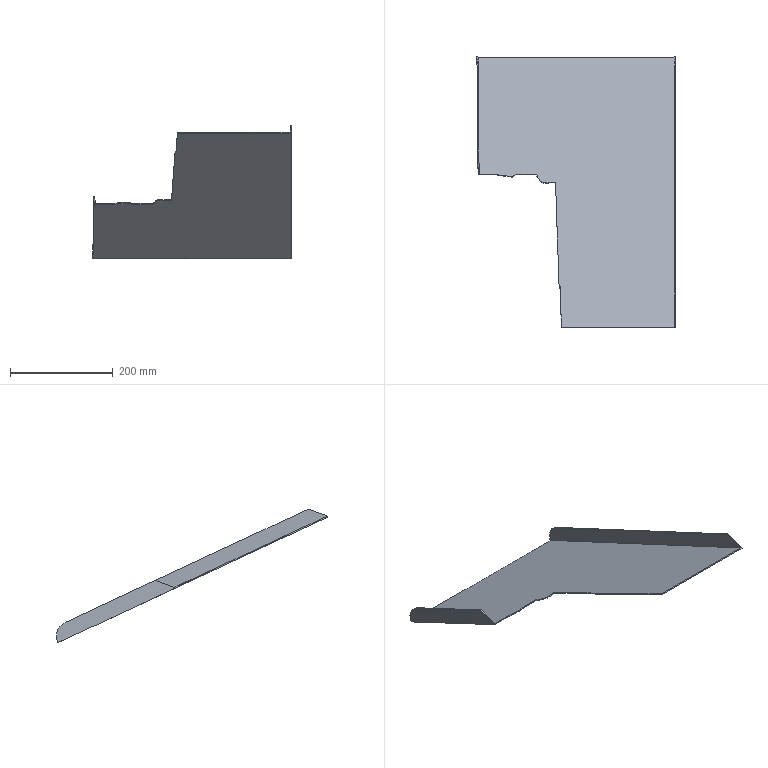Part | NX | features solid 2 | 1 solid | 23 faces | box 386.058 x 528.771 x 260.615 mm | volume 388760 mm3 | plane 16 | spline 5 | cylinder 2 | commonest cylinder face diameters 60 x2
STEP:
#1=CARTESIAN_POINT('',(1004.04,594.165,-105.));
#2=VERTEX_POINT('',#1);
#3=CARTESIAN_POINT('',(1004.172,589.433,-105.));
#4=VERTEX_POINT('',#3);
#5=CARTESIAN_POINT('',(1001.433,687.077,-105.));
#6=DIRECTION('',(0.02804,-0.9996,0.));
#7=VECTOR('',#6,1000.);
#8=LINE('',#5,#7);
#9=EDGE_CURVE('',#2,#4,#8,.T.);
#10=ORIENTED_EDGE('',*,*,#9,.F.);
#11=CARTESIAN_POINT('',(1000.877,686.781,-148.187));
#12=VERTEX_POINT('',#11);
#13=CARTESIAN_POINT('',(995.195,853.126,-225.756));
#14=DIRECTION('',(0.03094,-0.9059,0.4224));
#15=VECTOR('',#14,1000.);
#16=LINE('',#13,#15);
#17=EDGE_CURVE('',#12,#2,#16,.T.);
#18=ORIENTED_EDGE('',*,*,#17,.F.);
#19=CARTESIAN_POINT('',(1000.877,685.936,-150.));
#20=VERTEX_POINT('',#19);
#21=CARTESIAN_POINT('',(1000.877,686.781,-148.187));
#22=DIRECTION('',(0.,-0.4226,-0.9063));
#23=VECTOR('',#22,1000.);
#24=LINE('',#21,#23);
#25=EDGE_CURVE('',#12,#20,#24,.T.);
#26=ORIENTED_EDGE('',*,*,#25,.T.);
#27=CARTESIAN_POINT('',(995.195,852.281,-227.568));
#28=DIRECTION('',(0.03094,-0.9059,0.4224));
#29=VECTOR('',#28,1000.);
#30=LINE('',#27,#29);
#31=EDGE_CURVE('',#20,#4,#30,.T.);
#32=ORIENTED_EDGE('',*,*,#31,.T.);
#33=EDGE_LOOP('',(#10,#18,#26,#32));
#34=FACE_BOUND('',#33,.T.);
#35=CARTESIAN_POINT('',(1000.867,687.061,-148.318));
#36=DIRECTION('',(0.9995,0.02804,-0.01308));
#37=DIRECTION('',(-0.02804,0.9996,0.));
#38=AXIS2_PLACEMENT_3D('',#35,#36,#37);
#39=PLANE('',#38);
#40=ADVANCED_FACE('',(#34),#39,.F.);
#41=CARTESIAN_POINT('',(1228.,514.901,-68.039));
#42=VERTEX_POINT('',#41);
#43=CARTESIAN_POINT('',(1008.582,514.901,-68.039));
#44=VERTEX_POINT('',#43);
#45=CARTESIAN_POINT('',(885.33,514.901,-68.039));
#46=DIRECTION('',(-1.,0.,0.));
#47=VECTOR('',#46,1000.);
#48=LINE('',#45,#47);
#49=EDGE_CURVE('',#42,#44,#48,.T.);
#50=ORIENTED_EDGE('',*,*,#49,.F.);
#51=CARTESIAN_POINT('',(1228.,1040.,-312.896));
#52=VERTEX_POINT('',#51);
#53=CARTESIAN_POINT('',(1228.,850.044,-224.318));
#54=DIRECTION('',(0.,0.9063,-0.4226));
#55=VECTOR('',#54,1000.);
#56=LINE('',#53,#55);
#57=EDGE_CURVE('',#42,#52,#56,.T.);
#58=ORIENTED_EDGE('',*,*,#57,.T.);
#59=CARTESIAN_POINT('',(845.95,1040.,-312.896));
#60=VERTEX_POINT('',#59);
#61=CARTESIAN_POINT('',(1230.,1040.,-312.896));
#62=DIRECTION('',(1.,0.,0.));
#63=VECTOR('',#62,1000.);
#64=LINE('',#61,#63);
#65=EDGE_CURVE('',#60,#52,#64,.T.);
#66=ORIENTED_EDGE('',*,*,#65,.F.);
#67=CARTESIAN_POINT('',(848.131,813.26,-207.165));
#68=VERTEX_POINT('',#67);
#69=CARTESIAN_POINT('',(847.78,849.747,-224.18));
#70=DIRECTION('',(0.008719,-0.9063,0.4226));
#71=VECTOR('',#70,1000.);
#72=LINE('',#69,#71);
#73=EDGE_CURVE('',#60,#68,#72,.T.);
#74=ORIENTED_EDGE('',*,*,#73,.T.);
#75=CARTESIAN_POINT('',(846.131,813.244,-207.158));
#76=VERTEX_POINT('',#75);
#77=CARTESIAN_POINT('',(846.131,813.244,-207.158));
#78=DIRECTION('',(1.,0.007902,-0.003685));
#79=VECTOR('',#78,1000.);
#80=LINE('',#77,#79);
#81=EDGE_CURVE('',#68,#76,#80,.F.);
#82=ORIENTED_EDGE('',*,*,#81,.T.);
#83=CARTESIAN_POINT('',(919.718,812.718,-206.913));
#84=VERTEX_POINT('',#83);
#85=CARTESIAN_POINT('',(919.718,812.718,-206.913));
#86=CARTESIAN_POINT('',(918.571,811.794,-206.482));
#87=CARTESIAN_POINT('',(916.885,810.36,-205.813));
#88=CARTESIAN_POINT('',(914.265,808.946,-205.154));
#89=CARTESIAN_POINT('',(912.003,808.25,-204.829));
#90=CARTESIAN_POINT('',(909.648,808.163,-204.789));
#91=CARTESIAN_POINT('',(907.312,808.551,-204.97));
#92=CARTESIAN_POINT('',(905.019,809.072,-205.213));
#93=CARTESIAN_POINT('',(901.926,809.626,-205.471));
#94=CARTESIAN_POINT('',(898.039,810.216,-205.746));
#95=CARTESIAN_POINT('',(891.84,811.288,-206.246));
#96=CARTESIAN_POINT('',(884.08,812.541,-206.83));
#97=CARTESIAN_POINT('',(874.624,813.216,-207.145));
#98=CARTESIAN_POINT('',(865.12,813.183,-207.13));
#99=CARTESIAN_POINT('',(855.628,813.352,-207.208));
#100=CARTESIAN_POINT('',(849.297,813.263,-207.167));
#101=CARTESIAN_POINT('',(846.131,813.244,-207.158));
#102=B_SPLINE_CURVE_WITH_KNOTS('',3,(#85,#86,#87,#88,#89,#90,#91,#92,#93,#94,#95,#96,#97,#98,#99,#100,#101),.UNSPECIFIED.,.F.,.F.,(4,1,1,1,1,1,1,1,1,1,1,1,1,1,4),(0.,0.00457,0.006855,0.00914,0.01142,0.01371,0.01599,0.01828,0.02285,0.02742,0.03656,0.0457,0.05484,0.06398,0.07312),.UNSPECIFIED.);
#103=EDGE_CURVE('',#84,#76,#102,.T.);
#104=ORIENTED_EDGE('',*,*,#103,.F.);
#105=CARTESIAN_POINT('',(959.528,812.564,-206.841));
#106=VERTEX_POINT('',#105);
#107=CARTESIAN_POINT('',(959.528,812.564,-206.841));
#108=CARTESIAN_POINT('',(957.869,812.541,-206.83));
#109=CARTESIAN_POINT('',(954.551,812.482,-206.803));
#110=CARTESIAN_POINT('',(947.916,812.586,-206.851));
#111=CARTESIAN_POINT('',(941.281,812.586,-206.851));
#112=CARTESIAN_POINT('',(934.646,812.614,-206.864));
#113=CARTESIAN_POINT('',(928.011,812.752,-206.929));
#114=CARTESIAN_POINT('',(923.035,812.65,-206.881));
#115=CARTESIAN_POINT('',(919.718,812.718,-206.913));
#116=B_SPLINE_CURVE_WITH_KNOTS('',3,(#107,#108,#109,#110,#111,#112,#113,#114,#115),.UNSPECIFIED.,.F.,.F.,(4,1,1,1,1,1,4),(0.,0.004976,0.009953,0.01991,0.02488,0.02986,0.03981),.UNSPECIFIED.);
#117=EDGE_CURVE('',#106,#84,#116,.T.);
#118=ORIENTED_EDGE('',*,*,#117,.F.);
#119=CARTESIAN_POINT('',(997.156,797.748,-199.932));
#120=VERTEX_POINT('',#119);
#121=CARTESIAN_POINT('',(997.156,797.748,-199.932));
#122=CARTESIAN_POINT('',(995.198,797.617,-199.871));
#123=CARTESIAN_POINT('',(991.282,797.359,-199.751));
#124=CARTESIAN_POINT('',(985.407,796.95,-199.56));
#125=CARTESIAN_POINT('',(980.512,796.674,-199.431));
#126=CARTESIAN_POINT('',(976.601,796.245,-199.231));
#127=CARTESIAN_POINT('',(972.678,796.512,-199.356));
#128=CARTESIAN_POINT('',(969.145,798.316,-200.197));
#129=CARTESIAN_POINT('',(966.688,801.074,-201.483));
#130=CARTESIAN_POINT('',(965.204,803.341,-202.54));
#131=CARTESIAN_POINT('',(963.981,805.749,-203.663));
#132=CARTESIAN_POINT('',(962.396,807.968,-204.698));
#133=CARTESIAN_POINT('',(960.912,810.24,-205.757));
#134=CARTESIAN_POINT('',(959.995,811.792,-206.481));
#135=CARTESIAN_POINT('',(959.528,812.564,-206.841));
#136=B_SPLINE_CURVE_WITH_KNOTS('',3,(#121,#122,#123,#124,#125,#126,#127,#128,#129,#130,#131,#132,#133,#134,#135),.UNSPECIFIED.,.F.,.F.,(4,1,1,1,1,1,1,1,1,1,1,1,4),(0.1717,0.1776,0.1835,0.1894,0.1924,0.1953,0.2012,0.2041,0.2071,0.21,0.213,0.2159,0.2189),.UNSPECIFIED.);
#137=EDGE_CURVE('',#120,#106,#136,.T.);
#138=ORIENTED_EDGE('',*,*,#137,.F.);
#139=CARTESIAN_POINT('',(1000.78,686.781,-148.187));
#140=VERTEX_POINT('',#139);
#141=CARTESIAN_POINT('',(1000.78,686.781,-148.187));
#142=CARTESIAN_POINT('',(1000.149,705.275,-156.811));
#143=CARTESIAN_POINT('',(999.189,733.015,-169.747));
#144=CARTESIAN_POINT('',(997.983,770.004,-186.995));
#145=CARTESIAN_POINT('',(997.33,788.498,-195.619));
#146=CARTESIAN_POINT('',(997.156,797.748,-199.932));
#147=B_SPLINE_CURVE_WITH_KNOTS('',3,(#141,#142,#143,#144,#145,#146),.UNSPECIFIED.,.F.,.F.,(4,1,1,4),(0.3191,0.3804,0.411,0.4416),.UNSPECIFIED.);
#148=EDGE_CURVE('',#140,#120,#147,.T.);
#149=ORIENTED_EDGE('',*,*,#148,.F.);
#150=CARTESIAN_POINT('',(-663.007,686.781,-148.187));
#151=DIRECTION('',(1.,0.,0.));
#152=VECTOR('',#151,1000.);
#153=LINE('',#150,#152);
#154=EDGE_CURVE('',#140,#12,#153,.T.);
#155=ORIENTED_EDGE('',*,*,#154,.T.);
#156=ORIENTED_EDGE('',*,*,#17,.T.);
#157=CARTESIAN_POINT('',(1005.805,594.165,-105.));
#158=VERTEX_POINT('',#157);
#159=CARTESIAN_POINT('',(885.33,594.165,-105.));
#160=DIRECTION('',(-1.,0.,0.));
#161=VECTOR('',#160,1000.);
#162=LINE('',#159,#161);
#163=EDGE_CURVE('',#158,#2,#162,.T.);
#164=ORIENTED_EDGE('',*,*,#163,.F.);
#165=CARTESIAN_POINT('',(1005.805,594.165,-105.));
#166=CARTESIAN_POINT('',(1006.712,567.743,-92.679));
#167=CARTESIAN_POINT('',(1007.638,541.322,-80.359));
#168=CARTESIAN_POINT('',(1008.582,514.901,-68.039));
#169=B_SPLINE_CURVE_WITH_KNOTS('',3,(#165,#166,#167,#168),.UNSPECIFIED.,.F.,.F.,(4,4),(0.3214,0.4091),.UNSPECIFIED.);
#170=EDGE_CURVE('',#158,#44,#169,.T.);
#171=ORIENTED_EDGE('',*,*,#170,.T.);
#172=EDGE_LOOP('',(#50,#58,#66,#74,#82,#104,#118,#138,#149,#155,#156,#164,#171));
#173=FACE_BOUND('',#172,.T.);
#174=CARTESIAN_POINT('',(885.33,850.044,-224.318));
#175=DIRECTION('',(0.,-0.4226,-0.9063));
#176=DIRECTION('',(0.,0.9063,-0.4226));
#177=AXIS2_PLACEMENT_3D('',#174,#175,#176);
#178=PLANE('',#177);
#179=ADVANCED_FACE('',(#173),#178,.F.);
#180=CARTESIAN_POINT('',(845.942,1040.,-315.103));
#181=VERTEX_POINT('',#180);
#182=CARTESIAN_POINT('',(1228.,1040.,-315.103));
#183=VERTEX_POINT('',#182);
#184=CARTESIAN_POINT('',(1230.,1040.,-315.103));
#185=DIRECTION('',(1.,0.,0.));
#186=VECTOR('',#185,1000.);
#187=LINE('',#184,#186);
#188=EDGE_CURVE('',#181,#183,#187,.T.);
#189=ORIENTED_EDGE('',*,*,#188,.T.);
#190=CARTESIAN_POINT('',(1230.,1040.,-315.103));
#191=VERTEX_POINT('',#190);
#192=CARTESIAN_POINT('',(1230.,1040.,-315.103));
#193=DIRECTION('',(1.,0.,0.));
#194=VECTOR('',#193,1000.);
#195=LINE('',#192,#194);
#196=EDGE_CURVE('',#191,#183,#195,.F.);
#197=ORIENTED_EDGE('',*,*,#196,.F.);
#198=CARTESIAN_POINT('',(1230.,514.056,-69.851));
#199=VERTEX_POINT('',#198);
#200=CARTESIAN_POINT('',(1230.,849.199,-226.131));
#201=DIRECTION('',(0.,0.9063,-0.4226));
#202=VECTOR('',#201,1000.);
#203=LINE('',#200,#202);
#204=EDGE_CURVE('',#191,#199,#203,.F.);
#205=ORIENTED_EDGE('',*,*,#204,.T.);
#206=CARTESIAN_POINT('',(1013.343,514.056,-69.851));
#207=VERTEX_POINT('',#206);
#208=CARTESIAN_POINT('',(885.33,514.056,-69.851));
#209=DIRECTION('',(-1.,0.,0.));
#210=VECTOR('',#209,1000.);
#211=LINE('',#208,#210);
#212=EDGE_CURVE('',#199,#207,#211,.T.);
#213=ORIENTED_EDGE('',*,*,#212,.T.);
#214=CARTESIAN_POINT('',(1008.582,514.896,-70.243));
#215=VERTEX_POINT('',#214);
#216=CARTESIAN_POINT('',(820.678,548.028,-85.693));
#217=DIRECTION('',(0.9816,-0.1731,0.08071));
#218=VECTOR('',#217,1000.);
#219=LINE('',#216,#218);
#220=EDGE_CURVE('',#215,#207,#219,.T.);
#221=ORIENTED_EDGE('',*,*,#220,.F.);
#222=CARTESIAN_POINT('',(1005.968,589.433,-105.));
#223=VERTEX_POINT('',#222);
#224=CARTESIAN_POINT('',(1005.968,589.433,-105.));
#225=CARTESIAN_POINT('',(1006.822,564.587,-93.414));
#226=CARTESIAN_POINT('',(1007.695,539.741,-81.828));
#227=CARTESIAN_POINT('',(1008.582,514.896,-70.243));
#228=B_SPLINE_CURVE_WITH_KNOTS('',3,(#224,#225,#226,#227),.UNSPECIFIED.,.F.,.F.,(4,4),(0.,0.08228),.UNSPECIFIED.);
#229=EDGE_CURVE('',#223,#215,#228,.T.);
#230=ORIENTED_EDGE('',*,*,#229,.F.);
#231=CARTESIAN_POINT('',(885.33,589.433,-105.));
#232=DIRECTION('',(-1.,0.,0.));
#233=VECTOR('',#232,1000.);
#234=LINE('',#231,#233);
#235=EDGE_CURVE('',#223,#4,#234,.T.);
#236=ORIENTED_EDGE('',*,*,#235,.T.);
#237=ORIENTED_EDGE('',*,*,#31,.F.);
#238=CARTESIAN_POINT('',(1000.78,685.936,-150.));
#239=VERTEX_POINT('',#238);
#240=CARTESIAN_POINT('',(-663.007,685.936,-150.));
#241=DIRECTION('',(1.,0.,0.));
#242=VECTOR('',#241,1000.);
#243=LINE('',#240,#242);
#244=EDGE_CURVE('',#239,#20,#243,.T.);
#245=ORIENTED_EDGE('',*,*,#244,.F.);
#246=CARTESIAN_POINT('',(997.156,796.903,-201.745));
#247=VERTEX_POINT('',#246);
#248=CARTESIAN_POINT('',(1000.78,685.936,-150.));
#249=CARTESIAN_POINT('',(1000.149,704.429,-158.624));
#250=CARTESIAN_POINT('',(999.189,732.17,-171.559));
#251=CARTESIAN_POINT('',(997.983,769.159,-188.808));
#252=CARTESIAN_POINT('',(997.33,787.652,-197.431));
#253=CARTESIAN_POINT('',(997.156,796.903,-201.745));
#254=B_SPLINE_CURVE_WITH_KNOTS('',3,(#248,#249,#250,#251,#252,#253),.UNSPECIFIED.,.F.,.F.,(4,1,1,4),(0.272,0.3332,0.3639,0.3945),.UNSPECIFIED.);
#255=EDGE_CURVE('',#239,#247,#254,.T.);
#256=ORIENTED_EDGE('',*,*,#255,.T.);
#257=CARTESIAN_POINT('',(959.528,811.718,-208.653));
#258=VERTEX_POINT('',#257);
#259=CARTESIAN_POINT('',(997.156,796.903,-201.745));
#260=CARTESIAN_POINT('',(995.253,796.776,-201.686));
#261=CARTESIAN_POINT('',(991.449,796.525,-201.569));
#262=CARTESIAN_POINT('',(985.743,796.129,-201.384));
#263=CARTESIAN_POINT('',(980.984,795.854,-201.256));
#264=CARTESIAN_POINT('',(977.187,795.469,-201.076));
#265=CARTESIAN_POINT('',(974.322,795.465,-201.074));
#266=CARTESIAN_POINT('',(971.427,796.328,-201.477));
#267=CARTESIAN_POINT('',(968.071,798.334,-202.412));
#268=CARTESIAN_POINT('',(965.808,801.398,-203.841));
#269=CARTESIAN_POINT('',(964.289,804.256,-205.174));
#270=CARTESIAN_POINT('',(963.345,805.856,-205.92));
#271=CARTESIAN_POINT('',(962.222,807.365,-206.623));
#272=CARTESIAN_POINT('',(960.959,809.324,-207.537));
#273=CARTESIAN_POINT('',(960.01,810.923,-208.283));
#274=CARTESIAN_POINT('',(959.528,811.718,-208.653));
#275=B_SPLINE_CURVE_WITH_KNOTS('',3,(#259,#260,#261,#262,#263,#264,#265,#266,#267,#268,#269,#270,#271,#272,#273,#274),.UNSPECIFIED.,.F.,.F.,(4,1,1,1,1,1,1,1,1,1,1,1,1,4),(-0.005006,0.0007141,0.006434,0.01215,0.01501,0.01787,0.02073,0.02359,0.02931,0.03217,0.0336,0.03503,0.03789,0.04075),.UNSPECIFIED.);
#276=EDGE_CURVE('',#247,#258,#275,.T.);
#277=ORIENTED_EDGE('',*,*,#276,.T.);
#278=CARTESIAN_POINT('',(919.718,811.872,-208.725));
#279=VERTEX_POINT('',#278);
#280=CARTESIAN_POINT('',(959.528,811.718,-208.653));
#281=CARTESIAN_POINT('',(957.869,811.696,-208.643));
#282=CARTESIAN_POINT('',(954.551,811.637,-208.615));
#283=CARTESIAN_POINT('',(947.916,811.741,-208.664));
#284=CARTESIAN_POINT('',(941.281,811.741,-208.664));
#285=CARTESIAN_POINT('',(934.646,811.769,-208.677));
#286=CARTESIAN_POINT('',(928.011,811.907,-208.741));
#287=CARTESIAN_POINT('',(923.035,811.805,-208.694));
#288=CARTESIAN_POINT('',(919.718,811.872,-208.725));
#289=B_SPLINE_CURVE_WITH_KNOTS('',3,(#280,#281,#282,#283,#284,#285,#286,#287,#288),.UNSPECIFIED.,.F.,.F.,(4,1,1,1,1,1,4),(0.,0.004976,0.009953,0.01991,0.02488,0.02986,0.03981),.UNSPECIFIED.);
#290=EDGE_CURVE('',#258,#279,#289,.T.);
#291=ORIENTED_EDGE('',*,*,#290,.T.);
#292=CARTESIAN_POINT('',(846.131,812.399,-208.971));
#293=VERTEX_POINT('',#292);
#294=CARTESIAN_POINT('',(846.131,812.399,-208.971));
#295=CARTESIAN_POINT('',(849.278,812.418,-208.98));
#296=CARTESIAN_POINT('',(855.571,812.506,-209.021));
#297=CARTESIAN_POINT('',(865.009,812.339,-208.943));
#298=CARTESIAN_POINT('',(874.454,812.371,-208.958));
#299=CARTESIAN_POINT('',(882.3,811.833,-208.707));
#300=CARTESIAN_POINT('',(888.549,810.966,-208.303));
#301=CARTESIAN_POINT('',(893.21,810.207,-207.949));
#302=CARTESIAN_POINT('',(897.863,809.4,-207.572));
#303=CARTESIAN_POINT('',(901.756,808.806,-207.296));
#304=CARTESIAN_POINT('',(904.855,808.261,-207.041));
#305=CARTESIAN_POINT('',(907.156,807.744,-206.8));
#306=CARTESIAN_POINT('',(909.475,807.333,-206.609));
#307=CARTESIAN_POINT('',(912.65,807.395,-206.638));
#308=CARTESIAN_POINT('',(916.289,808.99,-207.381));
#309=CARTESIAN_POINT('',(918.552,810.934,-208.288));
#310=CARTESIAN_POINT('',(919.718,811.872,-208.725));
#311=B_SPLINE_CURVE_WITH_KNOTS('',3,(#294,#295,#296,#297,#298,#299,#300,#301,#302,#303,#304,#305,#306,#307,#308,#309,#310),.UNSPECIFIED.,.F.,.F.,(4,1,1,1,1,1,1,1,1,1,1,1,1,1,4),(0.3081,0.3176,0.327,0.3365,0.3459,0.3506,0.3553,0.3601,0.3648,0.3671,0.3695,0.3719,0.3742,0.3789,0.3837),.UNSPECIFIED.);
#312=EDGE_CURVE('',#279,#293,#311,.F.);
#313=ORIENTED_EDGE('',*,*,#312,.T.);
#314=CARTESIAN_POINT('',(843.942,1040.,-315.103));
#315=VERTEX_POINT('',#314);
#316=CARTESIAN_POINT('',(845.78,848.886,-225.985));
#317=DIRECTION('',(0.008719,-0.9063,0.4226));
#318=VECTOR('',#317,1000.);
#319=LINE('',#316,#318);
#320=EDGE_CURVE('',#293,#315,#319,.F.);
#321=ORIENTED_EDGE('',*,*,#320,.T.);
#322=CARTESIAN_POINT('',(845.942,1040.016,-315.11));
#323=VERTEX_POINT('',#322);
#324=CARTESIAN_POINT('',(843.942,1040.,-315.103));
#325=DIRECTION('',(1.,0.007902,-0.003685));
#326=VECTOR('',#325,1000.);
#327=LINE('',#324,#326);
#328=EDGE_CURVE('',#315,#323,#327,.T.);
#329=ORIENTED_EDGE('',*,*,#328,.T.);
#330=CARTESIAN_POINT('',(848.131,812.414,-208.978));
#331=DIRECTION('',(-0.008719,0.9063,-0.4226));
#332=VECTOR('',#331,1000.);
#333=LINE('',#330,#332);
#334=EDGE_CURVE('',#181,#323,#333,.T.);
#335=ORIENTED_EDGE('',*,*,#334,.F.);
#336=EDGE_LOOP('',(#189,#197,#205,#213,#221,#230,#236,#237,#245,#256,#277,#291,#313,#321,#329,#335));
#337=FACE_BOUND('',#336,.T.);
#338=CARTESIAN_POINT('',(885.33,849.199,-226.131));
#339=DIRECTION('',(0.,-0.4226,-0.9063));
#340=DIRECTION('',(0.,0.9063,-0.4226));
#341=AXIS2_PLACEMENT_3D('',#338,#339,#340);
#342=PLANE('',#341);
#343=ADVANCED_FACE('',(#337),#342,.T.);
#344=ORIENTED_EDGE('',*,*,#312,.F.);
#345=CARTESIAN_POINT('',(919.718,812.718,-206.913));
#346=DIRECTION('',(0.,-0.4226,-0.9063));
#347=VECTOR('',#346,1000.);
#348=LINE('',#345,#347);
#349=EDGE_CURVE('',#84,#279,#348,.T.);
#350=ORIENTED_EDGE('',*,*,#349,.F.);
#351=ORIENTED_EDGE('',*,*,#103,.T.);
#352=CARTESIAN_POINT('',(846.131,812.821,-208.064));
#353=DIRECTION('',(0.,-0.4226,-0.9063));
#354=VECTOR('',#353,1000.);
#355=LINE('',#352,#354);
#356=EDGE_CURVE('',#76,#293,#355,.T.);
#357=ORIENTED_EDGE('',*,*,#356,.T.);
#358=EDGE_LOOP('',(#344,#350,#351,#357));
#359=FACE_BOUND('',#358,.T.);
#360=CARTESIAN_POINT('',(846.131,813.244,-207.158));
#361=CARTESIAN_POINT('',(846.131,812.399,-208.971));
#362=CARTESIAN_POINT('',(846.952,813.249,-207.16));
#363=CARTESIAN_POINT('',(846.952,812.404,-208.973));
#364=CARTESIAN_POINT('',(847.967,813.256,-207.164));
#365=CARTESIAN_POINT('',(847.967,812.411,-208.976));
#366=CARTESIAN_POINT('',(849.222,813.266,-207.168));
#367=CARTESIAN_POINT('',(849.222,812.42,-208.981));
#368=CARTESIAN_POINT('',(849.709,813.269,-207.17));
#369=CARTESIAN_POINT('',(849.709,812.424,-208.983));
#370=CARTESIAN_POINT('',(850.186,813.273,-207.172));
#371=CARTESIAN_POINT('',(850.186,812.428,-208.985));
#372=CARTESIAN_POINT('',(850.769,813.278,-207.174));
#373=CARTESIAN_POINT('',(850.769,812.433,-208.987));
#374=CARTESIAN_POINT('',(852.215,813.289,-207.179));
#375=CARTESIAN_POINT('',(852.215,812.444,-208.992));
#376=CARTESIAN_POINT('',(853.793,813.299,-207.184));
#377=CARTESIAN_POINT('',(853.793,812.453,-208.996));
#378=CARTESIAN_POINT('',(855.206,813.302,-207.185));
#379=CARTESIAN_POINT('',(855.206,812.457,-208.998));
#380=CARTESIAN_POINT('',(856.258,813.301,-207.185));
#381=CARTESIAN_POINT('',(856.258,812.456,-208.997));
#382=CARTESIAN_POINT('',(857.709,813.291,-207.18));
#383=CARTESIAN_POINT('',(857.709,812.446,-208.993));
#384=CARTESIAN_POINT('',(859.553,813.274,-207.172));
#385=CARTESIAN_POINT('',(859.553,812.429,-208.985));
#386=CARTESIAN_POINT('',(861.785,813.249,-207.161));
#387=CARTESIAN_POINT('',(861.785,812.404,-208.973));
#388=CARTESIAN_POINT('',(863.648,813.23,-207.152));
#389=CARTESIAN_POINT('',(863.648,812.385,-208.964));
#390=CARTESIAN_POINT('',(864.898,813.218,-207.146));
#391=CARTESIAN_POINT('',(864.898,812.373,-208.959));
#392=CARTESIAN_POINT('',(865.395,813.214,-207.144));
#393=CARTESIAN_POINT('',(865.395,812.369,-208.957));
#394=CARTESIAN_POINT('',(865.706,813.212,-207.143));
#395=CARTESIAN_POINT('',(865.706,812.367,-208.956));
#396=CARTESIAN_POINT('',(866.358,813.207,-207.141));
#397=CARTESIAN_POINT('',(866.358,812.362,-208.954));
#398=CARTESIAN_POINT('',(867.257,813.201,-207.138));
#399=CARTESIAN_POINT('',(867.257,812.356,-208.951));
#400=CARTESIAN_POINT('',(868.918,813.189,-207.133));
#401=CARTESIAN_POINT('',(868.918,812.344,-208.945));
#402=CARTESIAN_POINT('',(871.765,813.184,-207.13));
#403=CARTESIAN_POINT('',(871.765,812.339,-208.943));
#404=CARTESIAN_POINT('',(876.169,813.072,-207.078));
#405=CARTESIAN_POINT('',(876.169,812.227,-208.891));
#406=CARTESIAN_POINT('',(880.461,812.783,-206.943));
#407=CARTESIAN_POINT('',(880.461,811.937,-208.756));
#408=CARTESIAN_POINT('',(883.49,812.472,-206.798));
#409=CARTESIAN_POINT('',(883.49,811.627,-208.611));
#410=CARTESIAN_POINT('',(884.822,812.313,-206.724));
#411=CARTESIAN_POINT('',(884.822,811.468,-208.537));
#412=CARTESIAN_POINT('',(885.507,812.226,-206.683));
#413=CARTESIAN_POINT('',(885.507,811.381,-208.496));
#414=CARTESIAN_POINT('',(885.787,812.19,-206.666));
#415=CARTESIAN_POINT('',(885.787,811.344,-208.479));
#416=CARTESIAN_POINT('',(886.311,812.12,-206.634));
#417=CARTESIAN_POINT('',(886.311,811.274,-208.446));
#418=CARTESIAN_POINT('',(887.113,812.007,-206.581));
#419=CARTESIAN_POINT('',(887.113,811.162,-208.394));
#420=CARTESIAN_POINT('',(888.532,811.798,-206.484));
#421=CARTESIAN_POINT('',(888.532,810.952,-208.296));
#422=CARTESIAN_POINT('',(890.577,811.479,-206.335));
#423=CARTESIAN_POINT('',(890.577,810.633,-208.148));
#424=CARTESIAN_POINT('',(892.915,811.096,-206.156));
#425=CARTESIAN_POINT('',(892.915,810.25,-207.969));
#426=CARTESIAN_POINT('',(895.127,810.721,-205.982));
#427=CARTESIAN_POINT('',(895.127,809.876,-207.794));
#428=CARTESIAN_POINT('',(896.541,810.481,-205.87));
#429=CARTESIAN_POINT('',(896.541,809.636,-207.682));
#430=CARTESIAN_POINT('',(897.813,810.269,-205.771));
#431=CARTESIAN_POINT('',(897.813,809.424,-207.584));
#432=CARTESIAN_POINT('',(898.77,810.113,-205.698));
#433=CARTESIAN_POINT('',(898.77,809.268,-207.511));
#434=CARTESIAN_POINT('',(899.361,810.018,-205.654));
#435=CARTESIAN_POINT('',(899.361,809.173,-207.467));
#436=CARTESIAN_POINT('',(899.71,809.963,-205.628));
#437=CARTESIAN_POINT('',(899.71,809.118,-207.441));
#438=CARTESIAN_POINT('',(899.884,809.936,-205.615));
#439=CARTESIAN_POINT('',(899.884,809.091,-207.428));
#440=CARTESIAN_POINT('',(900.35,809.863,-205.582));
#441=CARTESIAN_POINT('',(900.35,809.018,-207.394));
#442=CARTESIAN_POINT('',(900.891,809.777,-205.542));
#443=CARTESIAN_POINT('',(900.891,808.932,-207.354));
#444=CARTESIAN_POINT('',(901.812,809.629,-205.473));
#445=CARTESIAN_POINT('',(901.812,808.784,-207.285));
#446=CARTESIAN_POINT('',(902.962,809.438,-205.383));
#447=CARTESIAN_POINT('',(902.962,808.593,-207.196));
#448=CARTESIAN_POINT('',(903.916,809.269,-205.305));
#449=CARTESIAN_POINT('',(903.916,808.424,-207.117));
#450=CARTESIAN_POINT('',(904.586,809.142,-205.245));
#451=CARTESIAN_POINT('',(904.586,808.297,-207.058));
#452=CARTESIAN_POINT('',(905.004,809.057,-205.206));
#453=CARTESIAN_POINT('',(905.004,808.212,-207.018));
#454=CARTESIAN_POINT('',(905.661,808.92,-205.142));
#455=CARTESIAN_POINT('',(905.661,808.075,-206.954));
#456=CARTESIAN_POINT('',(906.44,808.758,-205.066));
#457=CARTESIAN_POINT('',(906.44,807.913,-206.879));
#458=CARTESIAN_POINT('',(907.325,808.569,-204.978));
#459=CARTESIAN_POINT('',(907.325,807.723,-206.791));
#460=CARTESIAN_POINT('',(907.842,808.47,-204.932));
#461=CARTESIAN_POINT('',(907.842,807.625,-206.745));
#462=CARTESIAN_POINT('',(908.47,808.368,-204.884));
#463=CARTESIAN_POINT('',(908.47,807.523,-206.697));
#464=CARTESIAN_POINT('',(909.354,808.256,-204.832));
#465=CARTESIAN_POINT('',(909.354,807.411,-206.645));
#466=CARTESIAN_POINT('',(910.417,808.194,-204.803));
#467=CARTESIAN_POINT('',(910.417,807.349,-206.616));
#468=CARTESIAN_POINT('',(911.708,808.264,-204.836));
#469=CARTESIAN_POINT('',(911.708,807.419,-206.648));
#470=CARTESIAN_POINT('',(913.182,808.599,-204.992));
#471=CARTESIAN_POINT('',(913.182,807.754,-206.805));
#472=CARTESIAN_POINT('',(914.316,809.028,-205.192));
#473=CARTESIAN_POINT('',(914.316,808.182,-207.005));
#474=CARTESIAN_POINT('',(915.131,809.43,-205.379));
#475=CARTESIAN_POINT('',(915.131,808.584,-207.192));
#476=CARTESIAN_POINT('',(915.571,809.665,-205.489));
#477=CARTESIAN_POINT('',(915.571,808.82,-207.302));
#478=CARTESIAN_POINT('',(916.357,810.13,-205.706));
#479=CARTESIAN_POINT('',(916.357,809.284,-207.518));
#480=CARTESIAN_POINT('',(917.318,810.802,-206.019));
#481=CARTESIAN_POINT('',(917.318,809.956,-207.832));
#482=CARTESIAN_POINT('',(918.158,811.461,-206.327));
#483=CARTESIAN_POINT('',(918.158,810.616,-208.139));
#484=CARTESIAN_POINT('',(918.858,812.026,-206.59));
#485=CARTESIAN_POINT('',(918.858,811.181,-208.403));
#486=CARTESIAN_POINT('',(919.372,812.44,-206.783));
#487=CARTESIAN_POINT('',(919.372,811.594,-208.596));
#488=CARTESIAN_POINT('',(919.718,812.718,-206.913));
#489=CARTESIAN_POINT('',(919.718,811.872,-208.725));
#490=B_SPLINE_SURFACE_WITH_KNOTS('',3,1,((#360,#361),(#362,#363),(#364,#365),(#366,#367),(#368,#369),(#370,#371),(#372,#373),(#374,#375),(#376,#377),(#378,#379),(#380,#381),(#382,#383),(#384,#385),(#386,#387),(#388,#389),(#390,#391),(#392,#393),(#394,#395),(#396,#397),(#398,#399),(#400,#401),(#402,#403),(#404,#405),(#406,#407),(#408,#409),(#410,#411),(#412,#413),(#414,#415),(#416,#417),(#418,#419),(#420,#421),(#422,#423),(#424,#425),(#426,#427),(#428,#429),(#430,#431),(#432,#433),(#434,#435),(#436,#437),(#438,#439),(#440,#441),(#442,#443),(#444,#445),(#446,#447),(#448,#449),(#450,#451),(#452,#453),(#454,#455),(#456,#457),(#458,#459),(#460,#461),(#462,#463),(#464,#465),(#466,#467),(#468,#469),(#470,#471),(#472,#473),(#474,#475),(#476,#477),(#478,#479),(#480,#481),(#482,#483),(#484,#485),(#486,#487),(#488,#489)),.SURF_OF_LINEAR_EXTRUSION.,.F.,.F.,.F.,(4,1,1,1,1,1,1,1,1,1,1,1,1,1,1,1,1,1,1,1,1,1,1,1,1,1,1,1,1,1,1,1,1,1,1,1,1,1,1,1,1,1,1,1,1,1,1,1,1,1,1,1,1,1,1,1,1,1,1,1,1,1,4),(2,2),(-0.0001288,0.03183,0.03982,0.04781,0.05181,0.0558,0.0638,0.09576,0.1117,0.1277,0.1597,0.1757,0.1916,0.2236,0.2396,0.2476,0.2516,0.2556,0.2715,0.2875,0.3195,0.3834,0.4473,0.4793,0.4953,0.4993,0.5033,0.5113,0.5272,0.5432,0.5752,0.6071,0.6231,0.6391,0.6551,0.6711,0.6791,0.6831,0.6871,0.691,0.695,0.703,0.719,0.735,0.743,0.751,0.759,0.767,0.7829,0.7909,0.7989,0.8149,0.8309,0.8628,0.8948,0.9268,0.9348,0.9428,0.9587,0.9907,0.9987,1.007,1.023),(0.,1.),.UNSPECIFIED.);
#491=ADVANCED_FACE('',(#359),#490,.F.);
#492=ORIENTED_EDGE('',*,*,#290,.F.);
#493=CARTESIAN_POINT('',(959.528,812.564,-206.841));
#494=DIRECTION('',(0.,-0.4226,-0.9063));
#495=VECTOR('',#494,1000.);
#496=LINE('',#493,#495);
#497=EDGE_CURVE('',#106,#258,#496,.T.);
#498=ORIENTED_EDGE('',*,*,#497,.F.);
#499=ORIENTED_EDGE('',*,*,#117,.T.);
#500=ORIENTED_EDGE('',*,*,#349,.T.);
#501=EDGE_LOOP('',(#492,#498,#499,#500));
#502=FACE_BOUND('',#501,.T.);
#503=CARTESIAN_POINT('',(919.718,812.718,-206.913));
#504=CARTESIAN_POINT('',(919.718,811.872,-208.725));
#505=CARTESIAN_POINT('',(920.208,812.708,-206.908));
#506=CARTESIAN_POINT('',(920.208,811.863,-208.721));
#507=CARTESIAN_POINT('',(920.807,812.696,-206.902));
#508=CARTESIAN_POINT('',(920.807,811.85,-208.715));
#509=CARTESIAN_POINT('',(921.567,812.68,-206.895));
#510=CARTESIAN_POINT('',(921.567,811.835,-208.708));
#511=CARTESIAN_POINT('',(921.988,812.672,-206.891));
#512=CARTESIAN_POINT('',(921.988,811.827,-208.704));
#513=CARTESIAN_POINT('',(922.777,812.668,-206.89));
#514=CARTESIAN_POINT('',(922.777,811.823,-208.702));
#515=CARTESIAN_POINT('',(923.866,812.675,-206.893));
#516=CARTESIAN_POINT('',(923.866,811.83,-208.705));
#517=CARTESIAN_POINT('',(924.794,812.685,-206.898));
#518=CARTESIAN_POINT('',(924.794,811.84,-208.71));
#519=CARTESIAN_POINT('',(925.349,812.693,-206.901));
#520=CARTESIAN_POINT('',(925.349,811.847,-208.714));
#521=CARTESIAN_POINT('',(926.003,812.702,-206.906));
#522=CARTESIAN_POINT('',(926.003,811.857,-208.718));
#523=CARTESIAN_POINT('',(926.38,812.707,-206.908));
#524=CARTESIAN_POINT('',(926.38,811.862,-208.72));
#525=CARTESIAN_POINT('',(927.238,812.712,-206.91));
#526=CARTESIAN_POINT('',(927.238,811.867,-208.723));
#527=CARTESIAN_POINT('',(928.321,812.71,-206.909));
#528=CARTESIAN_POINT('',(928.321,811.865,-208.722));
#529=CARTESIAN_POINT('',(929.542,812.698,-206.903));
#530=CARTESIAN_POINT('',(929.542,811.853,-208.716));
#531=CARTESIAN_POINT('',(930.587,812.681,-206.896));
#532=CARTESIAN_POINT('',(930.587,811.836,-208.708));
#533=CARTESIAN_POINT('',(931.396,812.668,-206.89));
#534=CARTESIAN_POINT('',(931.396,811.823,-208.702));
#535=CARTESIAN_POINT('',(932.49,812.653,-206.882));
#536=CARTESIAN_POINT('',(932.49,811.807,-208.695));
#537=CARTESIAN_POINT('',(933.772,812.637,-206.875));
#538=CARTESIAN_POINT('',(933.772,811.791,-208.688));
#539=CARTESIAN_POINT('',(935.065,812.623,-206.869));
#540=CARTESIAN_POINT('',(935.065,811.778,-208.681));
#541=CARTESIAN_POINT('',(936.36,812.612,-206.863));
#542=CARTESIAN_POINT('',(936.36,811.767,-208.676));
#543=CARTESIAN_POINT('',(937.44,812.605,-206.86));
#544=CARTESIAN_POINT('',(937.44,811.76,-208.673));
#545=CARTESIAN_POINT('',(938.201,812.601,-206.858));
#546=CARTESIAN_POINT('',(938.201,811.756,-208.671));
#547=CARTESIAN_POINT('',(938.629,812.599,-206.857));
#548=CARTESIAN_POINT('',(938.629,811.754,-208.67));
#549=CARTESIAN_POINT('',(938.914,812.598,-206.857));
#550=CARTESIAN_POINT('',(938.914,811.753,-208.669));
#551=CARTESIAN_POINT('',(939.103,812.597,-206.857));
#552=CARTESIAN_POINT('',(939.103,811.752,-208.669));
#553=CARTESIAN_POINT('',(939.59,812.595,-206.856));
#554=CARTESIAN_POINT('',(939.59,811.75,-208.668));
#555=CARTESIAN_POINT('',(940.279,812.593,-206.855));
#556=CARTESIAN_POINT('',(940.279,811.748,-208.667));
#557=CARTESIAN_POINT('',(941.674,812.588,-206.852));
#558=CARTESIAN_POINT('',(941.674,811.743,-208.665));
#559=CARTESIAN_POINT('',(943.375,812.582,-206.849));
#560=CARTESIAN_POINT('',(943.375,811.736,-208.662));
#561=CARTESIAN_POINT('',(945.055,812.576,-206.846));
#562=CARTESIAN_POINT('',(945.055,811.73,-208.659));
#563=CARTESIAN_POINT('',(946.343,812.571,-206.844));
#564=CARTESIAN_POINT('',(946.343,811.726,-208.657));
#565=CARTESIAN_POINT('',(947.257,812.567,-206.843));
#566=CARTESIAN_POINT('',(947.257,811.722,-208.655));
#567=CARTESIAN_POINT('',(947.678,812.566,-206.842));
#568=CARTESIAN_POINT('',(947.678,811.721,-208.655));
#569=CARTESIAN_POINT('',(947.847,812.565,-206.842));
#570=CARTESIAN_POINT('',(947.847,811.72,-208.654));
#571=CARTESIAN_POINT('',(947.834,812.565,-206.842));
#572=CARTESIAN_POINT('',(947.834,811.72,-208.654));
#573=CARTESIAN_POINT('',(947.915,812.565,-206.841));
#574=CARTESIAN_POINT('',(947.915,811.72,-208.654));
#575=CARTESIAN_POINT('',(948.167,812.563,-206.841));
#576=CARTESIAN_POINT('',(948.167,811.718,-208.653));
#577=CARTESIAN_POINT('',(948.424,812.561,-206.84));
#578=CARTESIAN_POINT('',(948.424,811.716,-208.652));
#579=CARTESIAN_POINT('',(948.867,812.558,-206.838));
#580=CARTESIAN_POINT('',(948.867,811.712,-208.651));
#581=CARTESIAN_POINT('',(949.628,812.551,-206.835));
#582=CARTESIAN_POINT('',(949.628,811.706,-208.648));
#583=CARTESIAN_POINT('',(950.723,812.541,-206.83));
#584=CARTESIAN_POINT('',(950.723,811.696,-208.643));
#585=CARTESIAN_POINT('',(952.466,812.521,-206.821));
#586=CARTESIAN_POINT('',(952.466,811.675,-208.633));
#587=CARTESIAN_POINT('',(954.677,812.501,-206.812));
#588=CARTESIAN_POINT('',(954.677,811.656,-208.624));
#589=CARTESIAN_POINT('',(957.055,812.53,-206.825));
#590=CARTESIAN_POINT('',(957.055,811.684,-208.638));
#591=CARTESIAN_POINT('',(958.709,812.553,-206.836));
#592=CARTESIAN_POINT('',(958.709,811.707,-208.648));
#593=CARTESIAN_POINT('',(959.528,812.564,-206.841));
#594=CARTESIAN_POINT('',(959.528,811.718,-208.653));
#595=B_SPLINE_SURFACE_WITH_KNOTS('',3,1,((#503,#504),(#505,#506),(#507,#508),(#509,#510),(#511,#512),(#513,#514),(#515,#516),(#517,#518),(#519,#520),(#521,#522),(#523,#524),(#525,#526),(#527,#528),(#529,#530),(#531,#532),(#533,#534),(#535,#536),(#537,#538),(#539,#540),(#541,#542),(#543,#544),(#545,#546),(#547,#548),(#549,#550),(#551,#552),(#553,#554),(#555,#556),(#557,#558),(#559,#560),(#561,#562),(#563,#564),(#565,#566),(#567,#568),(#569,#570),(#571,#572),(#573,#574),(#575,#576),(#577,#578),(#579,#580),(#581,#582),(#583,#584),(#585,#586),(#587,#588),(#589,#590),(#591,#592),(#593,#594)),.SURF_OF_LINEAR_EXTRUSION.,.F.,.F.,.F.,(4,1,1,1,1,1,1,1,1,1,1,1,1,1,1,1,1,1,1,1,1,1,1,1,1,1,1,1,1,1,1,1,1,1,1,1,1,1,1,1,1,1,1,4),(2,2),(-0.09934,-0.02493,-0.006328,0.01227,0.04948,0.08668,0.1053,0.1146,0.1239,0.1425,0.1611,0.1983,0.2355,0.2541,0.2727,0.3099,0.3471,0.3843,0.4215,0.4587,0.4773,0.4866,0.4959,0.5006,0.5052,0.5145,0.5331,0.5703,0.6075,0.6447,0.6819,0.7191,0.7377,0.747,0.7517,0.7563,0.7656,0.7749,0.7935,0.8307,0.8679,0.9423,1.017,1.091),(0.,1.),.UNSPECIFIED.);
#596=ADVANCED_FACE('',(#502),#595,.F.);
#597=ORIENTED_EDGE('',*,*,#276,.F.);
#598=CARTESIAN_POINT('',(997.156,797.325,-200.839));
#599=DIRECTION('',(0.,-0.4226,-0.9063));
#600=VECTOR('',#599,1000.);
#601=LINE('',#598,#600);
#602=EDGE_CURVE('',#120,#247,#601,.T.);
#603=ORIENTED_EDGE('',*,*,#602,.F.);
#604=ORIENTED_EDGE('',*,*,#137,.T.);
#605=ORIENTED_EDGE('',*,*,#497,.T.);
#606=EDGE_LOOP('',(#597,#603,#604,#605));
#607=FACE_BOUND('',#606,.T.);
#608=CARTESIAN_POINT('',(959.528,812.564,-206.841));
#609=CARTESIAN_POINT('',(959.528,811.718,-208.653));
#610=CARTESIAN_POINT('',(959.796,812.122,-206.635));
#611=CARTESIAN_POINT('',(959.796,811.276,-208.447));
#612=CARTESIAN_POINT('',(960.33,811.243,-206.225));
#613=CARTESIAN_POINT('',(960.33,810.398,-208.038));
#614=CARTESIAN_POINT('',(961.006,810.117,-205.7));
#615=CARTESIAN_POINT('',(961.006,809.272,-207.513));
#616=CARTESIAN_POINT('',(961.483,809.356,-205.345));
#617=CARTESIAN_POINT('',(961.483,808.511,-207.158));
#618=CARTESIAN_POINT('',(961.866,808.769,-205.071));
#619=CARTESIAN_POINT('',(961.866,807.924,-206.884));
#620=CARTESIAN_POINT('',(962.155,808.343,-204.873));
#621=CARTESIAN_POINT('',(962.155,807.498,-206.685));
#622=CARTESIAN_POINT('',(962.417,807.971,-204.699));
#623=CARTESIAN_POINT('',(962.417,807.126,-206.512));
#624=CARTESIAN_POINT('',(962.61,807.701,-204.573));
#625=CARTESIAN_POINT('',(962.61,806.856,-206.386));
#626=CARTESIAN_POINT('',(962.942,807.241,-204.359));
#627=CARTESIAN_POINT('',(962.942,806.395,-206.171));
#628=CARTESIAN_POINT('',(963.201,806.871,-204.186));
#629=CARTESIAN_POINT('',(963.201,806.026,-205.999));
#630=CARTESIAN_POINT('',(963.449,806.503,-204.015));
#631=CARTESIAN_POINT('',(963.449,805.658,-205.828));
#632=CARTESIAN_POINT('',(963.675,806.14,-203.845));
#633=CARTESIAN_POINT('',(963.675,805.295,-205.658));
#634=CARTESIAN_POINT('',(963.977,805.624,-203.605));
#635=CARTESIAN_POINT('',(963.977,804.779,-205.418));
#636=CARTESIAN_POINT('',(964.338,804.986,-203.307));
#637=CARTESIAN_POINT('',(964.338,804.14,-205.12));
#638=CARTESIAN_POINT('',(964.732,804.274,-202.975));
#639=CARTESIAN_POINT('',(964.732,803.428,-204.788));
#640=CARTESIAN_POINT('',(964.978,803.83,-202.769));
#641=CARTESIAN_POINT('',(964.978,802.985,-204.581));
#642=CARTESIAN_POINT('',(965.275,803.313,-202.527));
#643=CARTESIAN_POINT('',(965.275,802.468,-204.34));
#644=CARTESIAN_POINT('',(965.555,802.849,-202.311));
#645=CARTESIAN_POINT('',(965.555,802.004,-204.124));
#646=CARTESIAN_POINT('',(965.74,802.554,-202.173));
#647=CARTESIAN_POINT('',(965.74,801.709,-203.986));
#648=CARTESIAN_POINT('',(966.126,801.957,-201.895));
#649=CARTESIAN_POINT('',(966.126,801.111,-203.707));
#650=CARTESIAN_POINT('',(966.692,801.16,-201.523));
#651=CARTESIAN_POINT('',(966.692,800.315,-203.336));
#652=CARTESIAN_POINT('',(967.62,800.009,-200.987));
#653=CARTESIAN_POINT('',(967.62,799.164,-202.799));
#654=CARTESIAN_POINT('',(969.11,798.586,-200.323));
#655=CARTESIAN_POINT('',(969.11,797.74,-202.135));
#656=CARTESIAN_POINT('',(970.759,797.55,-199.84));
#657=CARTESIAN_POINT('',(970.759,796.705,-201.652));
#658=CARTESIAN_POINT('',(972.561,796.836,-199.507));
#659=CARTESIAN_POINT('',(972.561,795.991,-201.32));
#660=CARTESIAN_POINT('',(974.038,796.483,-199.342));
#661=CARTESIAN_POINT('',(974.038,795.638,-201.155));
#662=CARTESIAN_POINT('',(974.922,796.367,-199.288));
#663=CARTESIAN_POINT('',(974.922,795.522,-201.101));
#664=CARTESIAN_POINT('',(975.585,796.327,-199.27));
#665=CARTESIAN_POINT('',(975.585,795.482,-201.082));
#666=CARTESIAN_POINT('',(976.181,796.32,-199.266));
#667=CARTESIAN_POINT('',(976.181,795.474,-201.079));
#668=CARTESIAN_POINT('',(976.636,796.329,-199.271));
#669=CARTESIAN_POINT('',(976.636,795.484,-201.083));
#670=CARTESIAN_POINT('',(977.139,796.358,-199.284));
#671=CARTESIAN_POINT('',(977.139,795.513,-201.097));
#672=CARTESIAN_POINT('',(977.158,796.36,-199.285));
#673=CARTESIAN_POINT('',(977.158,795.515,-201.098));
#674=CARTESIAN_POINT('',(977.347,796.373,-199.291));
#675=CARTESIAN_POINT('',(977.347,795.528,-201.104));
#676=CARTESIAN_POINT('',(977.81,796.409,-199.308));
#677=CARTESIAN_POINT('',(977.81,795.564,-201.121));
#678=CARTESIAN_POINT('',(978.6,796.472,-199.337));
#679=CARTESIAN_POINT('',(978.6,795.627,-201.15));
#680=CARTESIAN_POINT('',(979.536,796.549,-199.373));
#681=CARTESIAN_POINT('',(979.536,795.704,-201.186));
#682=CARTESIAN_POINT('',(980.069,796.592,-199.393));
#683=CARTESIAN_POINT('',(980.069,795.747,-201.206));
#684=CARTESIAN_POINT('',(981.134,796.676,-199.432));
#685=CARTESIAN_POINT('',(981.134,795.83,-201.245));
#686=CARTESIAN_POINT('',(982.402,796.762,-199.472));
#687=CARTESIAN_POINT('',(982.402,795.916,-201.285));
#688=CARTESIAN_POINT('',(984.623,796.91,-199.542));
#689=CARTESIAN_POINT('',(984.623,796.065,-201.354));
#690=CARTESIAN_POINT('',(987.333,797.092,-199.626));
#691=CARTESIAN_POINT('',(987.333,796.247,-201.439));
#692=CARTESIAN_POINT('',(991.704,797.384,-199.762));
#693=CARTESIAN_POINT('',(991.704,796.538,-201.575));
#694=CARTESIAN_POINT('',(994.974,797.602,-199.864));
#695=CARTESIAN_POINT('',(994.974,796.757,-201.677));
#696=CARTESIAN_POINT('',(997.156,797.748,-199.932));
#697=CARTESIAN_POINT('',(997.156,796.903,-201.745));
#698=B_SPLINE_SURFACE_WITH_KNOTS('',3,1,((#608,#609),(#610,#611),(#612,#613),(#614,#615),(#616,#617),(#618,#619),(#620,#621),(#622,#623),(#624,#625),(#626,#627),(#628,#629),(#630,#631),(#632,#633),(#634,#635),(#636,#637),(#638,#639),(#640,#641),(#642,#643),(#644,#645),(#646,#647),(#648,#649),(#650,#651),(#652,#653),(#654,#655),(#656,#657),(#658,#659),(#660,#661),(#662,#663),(#664,#665),(#666,#667),(#668,#669),(#670,#671),(#672,#673),(#674,#675),(#676,#677),(#678,#679),(#680,#681),(#682,#683),(#684,#685),(#686,#687),(#688,#689),(#690,#691),(#692,#693),(#694,#695),(#696,#697)),.SURF_OF_LINEAR_EXTRUSION.,.F.,.F.,.F.,(4,1,1,1,1,1,1,1,1,1,1,1,1,1,1,1,1,1,1,1,1,1,1,1,1,1,1,1,1,1,1,1,1,1,1,1,1,1,1,1,1,1,4),(2,2),(-0.07533,-0.03353,0.008277,0.02918,0.05008,0.07098,0.08143,0.09188,0.1023,0.1128,0.1232,0.1337,0.1546,0.1755,0.1859,0.1964,0.2173,0.2382,0.2486,0.2591,0.3009,0.3427,0.4263,0.5099,0.5935,0.6353,0.6771,0.698,0.7189,0.7398,0.7503,0.7555,0.7607,0.7816,0.8025,0.813,0.8234,0.8443,0.8861,0.9279,1.012,1.095,1.262),(0.,1.),.UNSPECIFIED.);
#699=ADVANCED_FACE('',(#607),#698,.F.);
#700=ORIENTED_EDGE('',*,*,#255,.F.);
#701=CARTESIAN_POINT('',(1000.78,686.781,-148.187));
#702=DIRECTION('',(0.,-0.4226,-0.9063));
#703=VECTOR('',#702,1000.);
#704=LINE('',#701,#703);
#705=EDGE_CURVE('',#140,#239,#704,.T.);
#706=ORIENTED_EDGE('',*,*,#705,.F.);
#707=ORIENTED_EDGE('',*,*,#148,.T.);
#708=ORIENTED_EDGE('',*,*,#602,.T.);
#709=EDGE_LOOP('',(#700,#706,#707,#708));
#710=FACE_BOUND('',#709,.T.);
#711=CARTESIAN_POINT('',(997.156,797.748,-199.932));
#712=CARTESIAN_POINT('',(997.156,796.903,-201.745));
#713=CARTESIAN_POINT('',(997.169,797.022,-199.593));
#714=CARTESIAN_POINT('',(997.169,796.176,-201.406));
#715=CARTESIAN_POINT('',(997.19,795.932,-199.085));
#716=CARTESIAN_POINT('',(997.19,795.086,-200.898));
#717=CARTESIAN_POINT('',(997.214,794.661,-198.493));
#718=CARTESIAN_POINT('',(997.214,793.815,-200.305));
#719=CARTESIAN_POINT('',(997.228,793.933,-198.153));
#720=CARTESIAN_POINT('',(997.228,793.088,-199.966));
#721=CARTESIAN_POINT('',(997.238,793.39,-197.9));
#722=CARTESIAN_POINT('',(997.238,792.545,-199.713));
#723=CARTESIAN_POINT('',(997.248,792.839,-197.643));
#724=CARTESIAN_POINT('',(997.248,791.994,-199.456));
#725=CARTESIAN_POINT('',(997.262,792.143,-197.319));
#726=CARTESIAN_POINT('',(997.262,791.298,-199.131));
#727=CARTESIAN_POINT('',(997.344,789.346,-196.015));
#728=CARTESIAN_POINT('',(997.344,788.501,-197.827));
#729=CARTESIAN_POINT('',(997.528,783.557,-193.315));
#730=CARTESIAN_POINT('',(997.528,782.711,-195.127));
#731=CARTESIAN_POINT('',(997.754,776.586,-190.064));
#732=CARTESIAN_POINT('',(997.754,775.741,-191.877));
#733=CARTESIAN_POINT('',(997.979,769.745,-186.874));
#734=CARTESIAN_POINT('',(997.979,768.9,-188.687));
#735=CARTESIAN_POINT('',(998.17,763.979,-184.186));
#736=CARTESIAN_POINT('',(998.17,763.134,-185.998));
#737=CARTESIAN_POINT('',(998.347,758.646,-181.699));
#738=CARTESIAN_POINT('',(998.347,757.8,-183.511));
#739=CARTESIAN_POINT('',(998.5,754.061,-179.561));
#740=CARTESIAN_POINT('',(998.5,753.216,-181.373));
#741=CARTESIAN_POINT('',(998.62,750.464,-177.884));
#742=CARTESIAN_POINT('',(998.62,749.619,-179.696));
#743=CARTESIAN_POINT('',(998.745,746.709,-176.132));
#744=CARTESIAN_POINT('',(998.745,745.864,-177.945));
#745=CARTESIAN_POINT('',(998.854,743.447,-174.611));
#746=CARTESIAN_POINT('',(998.854,742.602,-176.424));
#747=CARTESIAN_POINT('',(998.944,740.758,-173.357));
#748=CARTESIAN_POINT('',(998.944,739.913,-175.17));
#749=CARTESIAN_POINT('',(999.013,738.702,-172.399));
#750=CARTESIAN_POINT('',(999.013,737.857,-174.211));
#751=CARTESIAN_POINT('',(999.072,736.955,-171.584));
#752=CARTESIAN_POINT('',(999.072,736.11,-173.397));
#753=CARTESIAN_POINT('',(999.119,735.539,-170.924));
#754=CARTESIAN_POINT('',(999.119,734.694,-172.736));
#755=CARTESIAN_POINT('',(999.155,734.464,-170.422));
#756=CARTESIAN_POINT('',(999.155,733.618,-172.235));
#757=CARTESIAN_POINT('',(999.185,733.57,-170.005));
#758=CARTESIAN_POINT('',(999.185,732.724,-171.818));
#759=CARTESIAN_POINT('',(999.207,732.919,-169.702));
#760=CARTESIAN_POINT('',(999.207,732.074,-171.515));
#761=CARTESIAN_POINT('',(999.217,732.621,-169.563));
#762=CARTESIAN_POINT('',(999.217,731.775,-171.376));
#763=CARTESIAN_POINT('',(999.224,732.404,-169.462));
#764=CARTESIAN_POINT('',(999.224,731.559,-171.275));
#765=CARTESIAN_POINT('',(999.226,732.359,-169.441));
#766=CARTESIAN_POINT('',(999.226,731.514,-171.254));
#767=CARTESIAN_POINT('',(999.226,732.354,-169.439));
#768=CARTESIAN_POINT('',(999.226,731.509,-171.251));
#769=CARTESIAN_POINT('',(999.227,732.316,-169.421));
#770=CARTESIAN_POINT('',(999.227,731.471,-171.234));
#771=CARTESIAN_POINT('',(999.229,732.26,-169.395));
#772=CARTESIAN_POINT('',(999.229,731.415,-171.207));
#773=CARTESIAN_POINT('',(999.232,732.166,-169.351));
#774=CARTESIAN_POINT('',(999.232,731.32,-171.163));
#775=CARTESIAN_POINT('',(999.237,732.042,-169.293));
#776=CARTESIAN_POINT('',(999.237,731.197,-171.106));
#777=CARTESIAN_POINT('',(999.243,731.859,-169.208));
#778=CARTESIAN_POINT('',(999.243,731.014,-171.02));
#779=CARTESIAN_POINT('',(999.255,731.496,-169.038));
#780=CARTESIAN_POINT('',(999.255,730.651,-170.851));
#781=CARTESIAN_POINT('',(999.277,730.85,-168.737));
#782=CARTESIAN_POINT('',(999.277,730.005,-170.55));
#783=CARTESIAN_POINT('',(999.321,729.548,-168.13));
#784=CARTESIAN_POINT('',(999.321,728.703,-169.943));
#785=CARTESIAN_POINT('',(999.394,727.416,-167.136));
#786=CARTESIAN_POINT('',(999.394,726.57,-168.948));
#787=CARTESIAN_POINT('',(999.508,724.05,-165.566));
#788=CARTESIAN_POINT('',(999.508,723.205,-167.379));
#789=CARTESIAN_POINT('',(999.65,719.878,-163.621));
#790=CARTESIAN_POINT('',(999.65,719.032,-165.433));
#791=CARTESIAN_POINT('',(999.877,713.238,-160.524));
#792=CARTESIAN_POINT('',(999.877,712.392,-162.337));
#793=CARTESIAN_POINT('',(1000.229,702.931,-155.719));
#794=CARTESIAN_POINT('',(1000.229,702.086,-157.531));
#795=CARTESIAN_POINT('',(1000.585,692.503,-150.856));
#796=CARTESIAN_POINT('',(1000.585,691.658,-152.668));
#797=CARTESIAN_POINT('',(1000.78,686.781,-148.187));
#798=CARTESIAN_POINT('',(1000.78,685.936,-150.));
#799=B_SPLINE_SURFACE_WITH_KNOTS('',3,1,((#711,#712),(#713,#714),(#715,#716),(#717,#718),(#719,#720),(#721,#722),(#723,#724),(#725,#726),(#727,#728),(#729,#730),(#731,#732),(#733,#734),(#735,#736),(#737,#738),(#739,#740),(#741,#742),(#743,#744),(#745,#746),(#747,#748),(#749,#750),(#751,#752),(#753,#754),(#755,#756),(#757,#758),(#759,#760),(#761,#762),(#763,#764),(#765,#766),(#767,#768),(#769,#770),(#771,#772),(#773,#774),(#775,#776),(#777,#778),(#779,#780),(#781,#782),(#783,#784),(#785,#786),(#787,#788),(#789,#790),(#791,#792),(#793,#794),(#795,#796),(#797,#798)),.SURF_OF_LINEAR_EXTRUSION.,.F.,.F.,.F.,(4,1,1,1,1,1,1,1,1,1,1,1,1,1,1,1,1,1,1,1,1,1,1,1,1,1,1,1,1,1,1,1,1,1,1,1,1,1,1,1,1,4),(2,2),(-0.4083,-0.2321,-0.144,-0.09995,-0.0559,-0.01184,0.03221,0.1203,0.2084,0.2965,0.3406,0.3847,0.4287,0.4507,0.4728,0.4948,0.5168,0.5278,0.5389,0.5499,0.5554,0.5609,0.5664,0.5691,0.5705,0.5712,0.5719,0.5733,0.5746,0.5774,0.5829,0.5884,0.5939,0.6049,0.627,0.649,0.693,0.7371,0.7812,0.8252,0.9133,1.001),(0.,1.),.UNSPECIFIED.);
#800=ADVANCED_FACE('',(#710),#799,.F.);
#801=ORIENTED_EDGE('',*,*,#244,.T.);
#802=ORIENTED_EDGE('',*,*,#25,.F.);
#803=ORIENTED_EDGE('',*,*,#154,.F.);
#804=ORIENTED_EDGE('',*,*,#705,.T.);
#805=EDGE_LOOP('',(#801,#802,#803,#804));
#806=FACE_BOUND('',#805,.T.);
#807=CARTESIAN_POINT('',(-663.007,686.781,-148.187));
#808=DIRECTION('',(0.,0.9063,-0.4226));
#809=DIRECTION('',(0.,0.4226,0.9063));
#810=AXIS2_PLACEMENT_3D('',#807,#808,#809);
#811=PLANE('',#810);
#812=ADVANCED_FACE('',(#806),#811,.F.);
#813=CARTESIAN_POINT('',(1008.582,514.896,-68.051));
#814=VERTEX_POINT('',#813);
#815=CARTESIAN_POINT('',(995.434,517.214,-63.079));
#816=DIRECTION('',(-0.9229,0.1627,0.349));
#817=VECTOR('',#816,1000.);
#818=LINE('',#815,#817);
#819=EDGE_CURVE('',#207,#814,#818,.T.);
#820=ORIENTED_EDGE('',*,*,#819,.F.);
#821=ORIENTED_EDGE('',*,*,#212,.F.);
#822=CARTESIAN_POINT('',(1230.,514.901,-68.039));
#823=VERTEX_POINT('',#822);
#824=CARTESIAN_POINT('',(1230.,514.901,-68.039));
#825=DIRECTION('',(0.,-0.4226,-0.9063));
#826=VECTOR('',#825,1000.);
#827=LINE('',#824,#826);
#828=EDGE_CURVE('',#823,#199,#827,.T.);
#829=ORIENTED_EDGE('',*,*,#828,.F.);
#830=CARTESIAN_POINT('',(885.33,514.901,-68.039));
#831=DIRECTION('',(-1.,0.,0.));
#832=VECTOR('',#831,1000.);
#833=LINE('',#830,#832);
#834=EDGE_CURVE('',#823,#42,#833,.T.);
#835=ORIENTED_EDGE('',*,*,#834,.T.);
#836=ORIENTED_EDGE('',*,*,#49,.T.);
#837=CARTESIAN_POINT('',(1008.582,514.901,-68.039));
#838=CARTESIAN_POINT('',(1008.582,514.899,-68.043));
#839=CARTESIAN_POINT('',(1008.582,514.897,-68.047));
#840=CARTESIAN_POINT('',(1008.582,514.896,-68.051));
#841=B_SPLINE_CURVE_WITH_KNOTS('',3,(#837,#838,#839,#840),.UNSPECIFIED.,.F.,.F.,(4,4),(0.001799,0.001813),.UNSPECIFIED.);
#842=EDGE_CURVE('',#44,#814,#841,.T.);
#843=ORIENTED_EDGE('',*,*,#842,.T.);
#844=EDGE_LOOP('',(#820,#821,#829,#835,#836,#843));
#845=FACE_BOUND('',#844,.T.);
#846=CARTESIAN_POINT('',(993.151,514.901,-68.039));
#847=DIRECTION('',(0.,-0.9063,0.4226));
#848=DIRECTION('',(0.,-0.4226,-0.9063));
#849=AXIS2_PLACEMENT_3D('',#846,#847,#848);
#850=PLANE('',#849);
#851=ADVANCED_FACE('',(#845),#850,.T.);
#852=CARTESIAN_POINT('',(1230.,552.111,-54.495));
#853=VERTEX_POINT('',#852);
#854=CARTESIAN_POINT('',(1230.,514.901,-68.039));
#855=DIRECTION('',(0.,-0.9397,-0.342));
#856=VECTOR('',#855,1000.);
#857=LINE('',#854,#856);
#858=EDGE_CURVE('',#853,#823,#857,.T.);
#859=ORIENTED_EDGE('',*,*,#858,.T.);
#860=ORIENTED_EDGE('',*,*,#828,.T.);
#861=ORIENTED_EDGE('',*,*,#204,.F.);
#862=CARTESIAN_POINT('',(1230.,1025.489,-275.235));
#863=VERTEX_POINT('',#862);
#864=CARTESIAN_POINT('',(1230.,1012.811,-302.424));
#865=DIRECTION('',(-1.,0.,0.));
#866=DIRECTION('',(0.,-1.,0.));
#867=AXIS2_PLACEMENT_3D('',#864,#865,#866);
#868=CIRCLE('',#867,30.);
#869=EDGE_CURVE('',#191,#863,#868,.F.);
#870=ORIENTED_EDGE('',*,*,#869,.T.);
#871=CARTESIAN_POINT('',(1230.,1052.679,-287.914));
#872=DIRECTION('',(0.,-0.9063,0.4226));
#873=VECTOR('',#872,1000.);
#874=LINE('',#871,#873);
#875=EDGE_CURVE('',#863,#853,#874,.T.);
#876=ORIENTED_EDGE('',*,*,#875,.T.);
#877=EDGE_LOOP('',(#859,#860,#861,#870,#876));
#878=FACE_BOUND('',#877,.T.);
#879=CARTESIAN_POINT('',(1230.,850.044,-224.318));
#880=DIRECTION('',(1.,0.,0.));
#881=DIRECTION('',(0.,1.,0.));
#882=AXIS2_PLACEMENT_3D('',#879,#880,#881);
#883=PLANE('',#882);
#884=ADVANCED_FACE('',(#878),#883,.T.);
#885=ORIENTED_EDGE('',*,*,#65,.T.);
#886=CARTESIAN_POINT('',(1228.,1040.,-720.));
#887=DIRECTION('',(0.,0.,-1.));
#888=VECTOR('',#887,1000.);
#889=LINE('',#886,#888);
#890=EDGE_CURVE('',#52,#183,#889,.T.);
#891=ORIENTED_EDGE('',*,*,#890,.T.);
#892=ORIENTED_EDGE('',*,*,#188,.F.);
#893=CARTESIAN_POINT('',(844.455,1040.,-718.579));
#894=DIRECTION('',(0.003685,0.,1.));
#895=VECTOR('',#894,1000.);
#896=LINE('',#893,#895);
#897=EDGE_CURVE('',#181,#60,#896,.T.);
#898=ORIENTED_EDGE('',*,*,#897,.T.);
#899=EDGE_LOOP('',(#885,#891,#892,#898));
#900=FACE_BOUND('',#899,.T.);
#901=CARTESIAN_POINT('',(1230.,1040.,-720.));
#902=DIRECTION('',(0.,-1.,0.));
#903=DIRECTION('',(-1.,0.,0.));
#904=AXIS2_PLACEMENT_3D('',#901,#902,#903);
#905=PLANE('',#904);
#906=ADVANCED_FACE('',(#900),#905,.F.);
#907=ORIENTED_EDGE('',*,*,#320,.F.);
#908=ORIENTED_EDGE('',*,*,#356,.F.);
#909=CARTESIAN_POINT('',(845.887,850.453,-193.614));
#910=VERTEX_POINT('',#909);
#911=CARTESIAN_POINT('',(845.887,850.453,-193.614));
#912=DIRECTION('',(0.006166,-0.9397,-0.342));
#913=VECTOR('',#912,1000.);
#914=LINE('',#911,#913);
#915=EDGE_CURVE('',#76,#910,#914,.F.);
#916=ORIENTED_EDGE('',*,*,#915,.T.);
#917=CARTESIAN_POINT('',(844.203,1025.49,-275.236));
#918=VERTEX_POINT('',#917);
#919=CARTESIAN_POINT('',(846.131,825.077,-181.781));
#920=DIRECTION('',(-0.008719,0.9063,-0.4226));
#921=VECTOR('',#920,1000.);
#922=LINE('',#919,#921);
#923=EDGE_CURVE('',#910,#918,#922,.T.);
#924=ORIENTED_EDGE('',*,*,#923,.T.);
#925=CARTESIAN_POINT('',(844.203,1012.812,-302.425));
#926=DIRECTION('',(1.,0.007902,-0.003685));
#927=DIRECTION('',(-0.007902,1.,0.));
#928=AXIS2_PLACEMENT_3D('',#925,#926,#927);
#929=CIRCLE('',#928,30.);
#930=EDGE_CURVE('',#918,#315,#929,.F.);
#931=ORIENTED_EDGE('',*,*,#930,.T.);
#932=EDGE_LOOP('',(#907,#908,#916,#924,#931));
#933=FACE_BOUND('',#932,.T.);
#934=CARTESIAN_POINT('',(845.78,849.732,-224.173));
#935=DIRECTION('',(-1.,-0.007902,0.003685));
#936=DIRECTION('',(0.007902,-1.,0.));
#937=AXIS2_PLACEMENT_3D('',#934,#935,#936);
#938=PLANE('',#937);
#939=ADVANCED_FACE('',(#933),#938,.T.);
#940=ORIENTED_EDGE('',*,*,#163,.T.);
#941=ORIENTED_EDGE('',*,*,#9,.T.);
#942=ORIENTED_EDGE('',*,*,#235,.F.);
#943=CARTESIAN_POINT('',(1005.968,589.433,-105.));
#944=CARTESIAN_POINT('',(1005.914,591.01,-105.));
#945=CARTESIAN_POINT('',(1005.859,592.588,-105.));
#946=CARTESIAN_POINT('',(1005.805,594.165,-105.));
#947=B_SPLINE_CURVE_WITH_KNOTS('',3,(#943,#944,#945,#946),.UNSPECIFIED.,.F.,.F.,(4,4),(0.,0.004735),.UNSPECIFIED.);
#948=EDGE_CURVE('',#223,#158,#947,.T.);
#949=ORIENTED_EDGE('',*,*,#948,.T.);
#950=EDGE_LOOP('',(#940,#941,#942,#949));
#951=FACE_BOUND('',#950,.T.);
#952=CARTESIAN_POINT('',(-1097.567,-373.462,-105.));
#953=DIRECTION('',(0.,0.,1.));
#954=DIRECTION('',(1.,0.,0.));
#955=AXIS2_PLACEMENT_3D('',#952,#953,#954);
#956=PLANE('',#955);
#957=ADVANCED_FACE('',(#951),#956,.T.);
#958=ORIENTED_EDGE('',*,*,#819,.T.);
#959=CARTESIAN_POINT('',(1008.582,514.896,-69.553));
#960=DIRECTION('',(0.,0.,-1.));
#961=VECTOR('',#960,1000.);
#962=LINE('',#959,#961);
#963=EDGE_CURVE('',#814,#215,#962,.T.);
#964=ORIENTED_EDGE('',*,*,#963,.T.);
#965=ORIENTED_EDGE('',*,*,#220,.T.);
#966=EDGE_LOOP('',(#958,#964,#965));
#967=FACE_BOUND('',#966,.T.);
#968=CARTESIAN_POINT('',(1154.132,489.231,-72.067));
#969=DIRECTION('',(0.1736,0.9848,0.));
#970=DIRECTION('',(-0.9848,0.1736,0.));
#971=AXIS2_PLACEMENT_3D('',#968,#969,#970);
#972=PLANE('',#971);
#973=ADVANCED_FACE('',(#967),#972,.F.);
#974=ORIENTED_EDGE('',*,*,#842,.F.);
#975=ORIENTED_EDGE('',*,*,#170,.F.);
#976=ORIENTED_EDGE('',*,*,#948,.F.);
#977=ORIENTED_EDGE('',*,*,#229,.T.);
#978=ORIENTED_EDGE('',*,*,#963,.F.);
#979=EDGE_LOOP('',(#974,#975,#976,#977,#978));
#980=FACE_BOUND('',#979,.T.);
#981=CARTESIAN_POINT('',(1005.789,594.639,-83.262));
#982=CARTESIAN_POINT('',(1005.789,594.639,-106.213));
#983=CARTESIAN_POINT('',(1006.698,568.133,-77.757));
#984=CARTESIAN_POINT('',(1006.698,568.133,-100.707));
#985=CARTESIAN_POINT('',(1007.63,541.543,-72.665));
#986=CARTESIAN_POINT('',(1007.63,541.543,-95.615));
#987=CARTESIAN_POINT('',(1008.582,514.896,-67.902));
#988=CARTESIAN_POINT('',(1008.582,514.896,-90.852));
#989=B_SPLINE_SURFACE_WITH_KNOTS('',3,1,((#981,#982),(#983,#984),(#985,#986),(#987,#988)),.SURF_OF_LINEAR_EXTRUSION.,.F.,.F.,.F.,(4,4),(2,2),(0.7321,1.018),(0.,1.),.PIECEWISE_BEZIER_KNOTS.);
#990=ADVANCED_FACE('',(#980),#989,.F.);
#991=ORIENTED_EDGE('',*,*,#73,.F.);
#992=ORIENTED_EDGE('',*,*,#897,.F.);
#993=ORIENTED_EDGE('',*,*,#334,.T.);
#994=CARTESIAN_POINT('',(846.203,1025.506,-275.243));
#995=VERTEX_POINT('',#994);
#996=CARTESIAN_POINT('',(846.203,1012.828,-302.432));
#997=DIRECTION('',(1.,0.007902,-0.003685));
#998=DIRECTION('',(-0.007902,1.,0.));
#999=AXIS2_PLACEMENT_3D('',#996,#997,#998);
#1000=CIRCLE('',#999,30.);
#1001=EDGE_CURVE('',#323,#995,#1000,.T.);
#1002=ORIENTED_EDGE('',*,*,#1001,.T.);
#1003=CARTESIAN_POINT('',(847.887,850.469,-193.622));
#1004=VERTEX_POINT('',#1003);
#1005=CARTESIAN_POINT('',(848.131,825.093,-181.789));
#1006=DIRECTION('',(-0.008719,0.9063,-0.4226));
#1007=VECTOR('',#1006,1000.);
#1008=LINE('',#1005,#1007);
#1009=EDGE_CURVE('',#1004,#995,#1008,.T.);
#1010=ORIENTED_EDGE('',*,*,#1009,.F.);
#1011=CARTESIAN_POINT('',(848.14,811.931,-207.649));
#1012=DIRECTION('',(-0.006166,0.9397,0.342));
#1013=VECTOR('',#1012,1000.);
#1014=LINE('',#1011,#1013);
#1015=EDGE_CURVE('',#1004,#68,#1014,.F.);
#1016=ORIENTED_EDGE('',*,*,#1015,.T.);
#1017=EDGE_LOOP('',(#991,#992,#993,#1002,#1010,#1016));
#1018=FACE_BOUND('',#1017,.T.);
#1019=CARTESIAN_POINT('',(848.131,812.414,-208.978));
#1020=DIRECTION('',(1.,0.007902,-0.003685));
#1021=DIRECTION('',(-0.007902,1.,0.));
#1022=AXIS2_PLACEMENT_3D('',#1019,#1020,#1021);
#1023=PLANE('',#1022);
#1024=ADVANCED_FACE('',(#1018),#1023,.T.);
#1025=ORIENTED_EDGE('',*,*,#923,.F.);
#1026=CARTESIAN_POINT('',(845.887,850.453,-193.614));
#1027=DIRECTION('',(-1.,-0.007902,0.003685));
#1028=VECTOR('',#1027,1000.);
#1029=LINE('',#1026,#1028);
#1030=EDGE_CURVE('',#910,#1004,#1029,.F.);
#1031=ORIENTED_EDGE('',*,*,#1030,.T.);
#1032=ORIENTED_EDGE('',*,*,#1009,.T.);
#1033=CARTESIAN_POINT('',(844.203,1025.49,-275.236));
#1034=DIRECTION('',(1.,0.007902,-0.003685));
#1035=VECTOR('',#1034,1000.);
#1036=LINE('',#1033,#1035);
#1037=EDGE_CURVE('',#995,#918,#1036,.F.);
#1038=ORIENTED_EDGE('',*,*,#1037,.T.);
#1039=EDGE_LOOP('',(#1025,#1031,#1032,#1038));
#1040=FACE_BOUND('',#1039,.T.);
#1041=CARTESIAN_POINT('',(846.131,825.077,-181.781));
#1042=DIRECTION('',(0.,-0.4226,-0.9063));
#1043=DIRECTION('',(-0.008719,0.9063,-0.4226));
#1044=AXIS2_PLACEMENT_3D('',#1041,#1042,#1043);
#1045=PLANE('',#1044);
#1046=ADVANCED_FACE('',(#1040),#1045,.F.);
#1047=ORIENTED_EDGE('',*,*,#930,.F.);
#1048=ORIENTED_EDGE('',*,*,#1037,.F.);
#1049=ORIENTED_EDGE('',*,*,#1001,.F.);
#1050=ORIENTED_EDGE('',*,*,#328,.F.);
#1051=EDGE_LOOP('',(#1047,#1048,#1049,#1050));
#1052=FACE_BOUND('',#1051,.T.);
#1053=CARTESIAN_POINT('',(844.203,1012.812,-302.425));
#1054=DIRECTION('',(-1.,-0.007902,0.003685));
#1055=DIRECTION('',(0.007902,-1.,0.));
#1056=AXIS2_PLACEMENT_3D('',#1053,#1054,#1055);
#1057=CYLINDRICAL_SURFACE('',#1056,30.);
#1058=ADVANCED_FACE('',(#1052),#1057,.T.);
#1059=ORIENTED_EDGE('',*,*,#915,.F.);
#1060=ORIENTED_EDGE('',*,*,#81,.F.);
#1061=ORIENTED_EDGE('',*,*,#1015,.F.);
#1062=ORIENTED_EDGE('',*,*,#1030,.F.);
#1063=EDGE_LOOP('',(#1059,#1060,#1061,#1062));
#1064=FACE_BOUND('',#1063,.T.);
#1065=CARTESIAN_POINT('',(845.887,850.453,-193.614));
#1066=DIRECTION('',(-0.006166,0.342,-0.9397));
#1067=DIRECTION('',(0.,0.9397,0.342));
#1068=AXIS2_PLACEMENT_3D('',#1065,#1066,#1067);
#1069=PLANE('',#1068);
#1070=ADVANCED_FACE('',(#1064),#1069,.F.);
#1071=ORIENTED_EDGE('',*,*,#57,.F.);
#1072=CARTESIAN_POINT('',(1228.,552.111,-54.495));
#1073=VERTEX_POINT('',#1072);
#1074=CARTESIAN_POINT('',(1228.,899.17,71.824));
#1075=DIRECTION('',(0.,0.9397,0.342));
#1076=VECTOR('',#1075,1000.);
#1077=LINE('',#1074,#1076);
#1078=EDGE_CURVE('',#42,#1073,#1077,.T.);
#1079=ORIENTED_EDGE('',*,*,#1078,.T.);
#1080=CARTESIAN_POINT('',(1228.,1025.489,-275.235));
#1081=VERTEX_POINT('',#1080);
#1082=CARTESIAN_POINT('',(1228.,1052.679,-287.914));
#1083=DIRECTION('',(0.,-0.9063,0.4226));
#1084=VECTOR('',#1083,1000.);
#1085=LINE('',#1082,#1084);
#1086=EDGE_CURVE('',#1081,#1073,#1085,.T.);
#1087=ORIENTED_EDGE('',*,*,#1086,.F.);
#1088=CARTESIAN_POINT('',(1228.,1012.811,-302.424));
#1089=DIRECTION('',(-1.,0.,0.));
#1090=DIRECTION('',(0.,-1.,0.));
#1091=AXIS2_PLACEMENT_3D('',#1088,#1089,#1090);
#1092=CIRCLE('',#1091,30.);
#1093=EDGE_CURVE('',#1081,#183,#1092,.T.);
#1094=ORIENTED_EDGE('',*,*,#1093,.T.);
#1095=ORIENTED_EDGE('',*,*,#890,.F.);
#1096=EDGE_LOOP('',(#1071,#1079,#1087,#1094,#1095));
#1097=FACE_BOUND('',#1096,.T.);
#1098=CARTESIAN_POINT('',(1228.,1040.,-315.103));
#1099=DIRECTION('',(-1.,0.,0.));
#1100=DIRECTION('',(0.,-1.,0.));
#1101=AXIS2_PLACEMENT_3D('',#1098,#1099,#1100);
#1102=PLANE('',#1101);
#1103=ADVANCED_FACE('',(#1097),#1102,.T.);
#1104=ORIENTED_EDGE('',*,*,#1086,.T.);
#1105=CARTESIAN_POINT('',(1230.,552.111,-54.495));
#1106=DIRECTION('',(1.,0.,0.));
#1107=VECTOR('',#1106,1000.);
#1108=LINE('',#1105,#1107);
#1109=EDGE_CURVE('',#1073,#853,#1108,.T.);
#1110=ORIENTED_EDGE('',*,*,#1109,.T.);
#1111=ORIENTED_EDGE('',*,*,#875,.F.);
#1112=CARTESIAN_POINT('',(1230.,1025.489,-275.235));
#1113=DIRECTION('',(-1.,0.,0.));
#1114=VECTOR('',#1113,1000.);
#1115=LINE('',#1112,#1114);
#1116=EDGE_CURVE('',#863,#1081,#1115,.T.);
#1117=ORIENTED_EDGE('',*,*,#1116,.T.);
#1118=EDGE_LOOP('',(#1104,#1110,#1111,#1117));
#1119=FACE_BOUND('',#1118,.T.);
#1120=CARTESIAN_POINT('',(1230.,1052.679,-287.914));
#1121=DIRECTION('',(0.,-0.4226,-0.9063));
#1122=DIRECTION('',(0.,-0.9063,0.4226));
#1123=AXIS2_PLACEMENT_3D('',#1120,#1121,#1122);
#1124=PLANE('',#1123);
#1125=ADVANCED_FACE('',(#1119),#1124,.F.);
#1126=ORIENTED_EDGE('',*,*,#869,.F.);
#1127=ORIENTED_EDGE('',*,*,#196,.T.);
#1128=ORIENTED_EDGE('',*,*,#1093,.F.);
#1129=ORIENTED_EDGE('',*,*,#1116,.F.);
#1130=EDGE_LOOP('',(#1126,#1127,#1128,#1129));
#1131=FACE_BOUND('',#1130,.T.);
#1132=CARTESIAN_POINT('',(1230.,1012.811,-302.424));
#1133=DIRECTION('',(-1.,0.,0.));
#1134=DIRECTION('',(0.,-1.,0.));
#1135=AXIS2_PLACEMENT_3D('',#1132,#1133,#1134);
#1136=CYLINDRICAL_SURFACE('',#1135,30.);
#1137=ADVANCED_FACE('',(#1131),#1136,.T.);
#1138=ORIENTED_EDGE('',*,*,#858,.F.);
#1139=ORIENTED_EDGE('',*,*,#1109,.F.);
#1140=ORIENTED_EDGE('',*,*,#1078,.F.);
#1141=ORIENTED_EDGE('',*,*,#834,.F.);
#1142=EDGE_LOOP('',(#1138,#1139,#1140,#1141));
#1143=FACE_BOUND('',#1142,.T.);
#1144=CARTESIAN_POINT('',(1230.,514.901,-68.039));
#1145=DIRECTION('',(0.,-0.342,0.9397));
#1146=DIRECTION('',(0.,-0.9397,-0.342));
#1147=AXIS2_PLACEMENT_3D('',#1144,#1145,#1146);
#1148=PLANE('',#1147);
#1149=ADVANCED_FACE('',(#1143),#1148,.T.);
#1150=CLOSED_SHELL('',(#40,#179,#343,#491,#596,#699,#800,#812,#851,#884,#906,#939,#957,#973,#990,#1024,#1046,#1058,#1070,#1103,#1125,#1137,#1149));
#1151=MANIFOLD_SOLID_BREP('',#1150);
#1152=(LENGTH_UNIT()NAMED_UNIT(*)SI_UNIT(.MILLI.,.METRE.));
#1153=UNCERTAINTY_MEASURE_WITH_UNIT(LENGTH_MEASURE(0.0508),#1152,'','');
#1154=(NAMED_UNIT(*)PLANE_ANGLE_UNIT()SI_UNIT($,.RADIAN.));
#1155=(NAMED_UNIT(*)SI_UNIT($,.STERADIAN.)SOLID_ANGLE_UNIT());
#1156=(GEOMETRIC_REPRESENTATION_CONTEXT(3)GLOBAL_UNCERTAINTY_ASSIGNED_CONTEXT((#1153))GLOBAL_UNIT_ASSIGNED_CONTEXT((#1152,#1154,#1155))REPRESENTATION_CONTEXT('',''));
#1157=ADVANCED_BREP_SHAPE_REPRESENTATION('',(#1151),#1156);